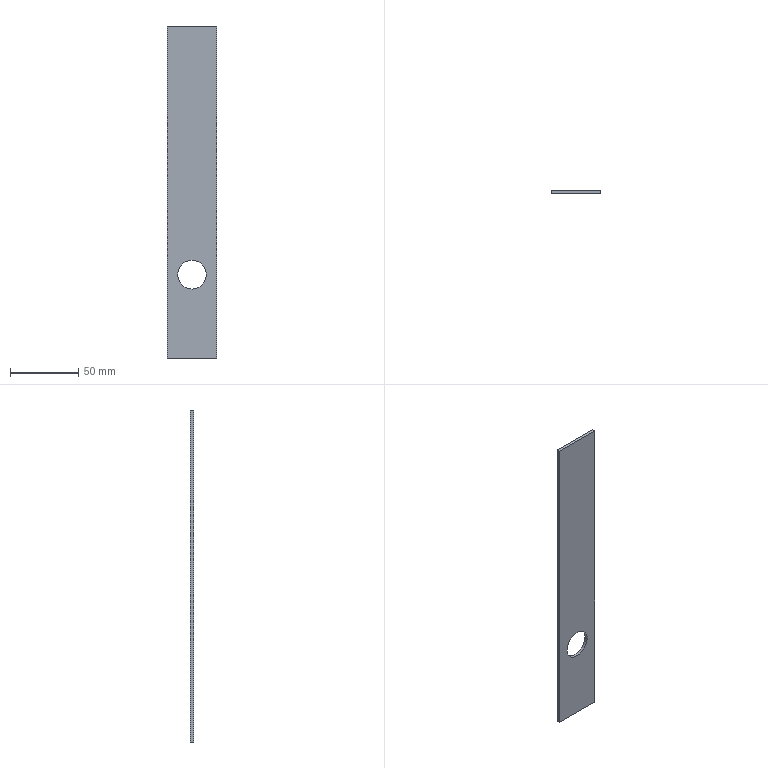Part | SolidWorks | features FlatPattern 1, SMBaseFlange 1, SheetMetal 1 | 1 solid | 8 faces | box 36.4 x 2.3 x 243 mm | volume 19547 mm3 | plane 6 | cylinder 2 | commonest cylinder face diameters 21 x2
STEP:
#1=CARTESIAN_POINT('',(0.,2.3,-71.));
#2=VERTEX_POINT('',#1);
#3=CARTESIAN_POINT('',(0.,2.3,-50.));
#4=VERTEX_POINT('',#3);
#5=CARTESIAN_POINT('',(0.,2.3,-60.5));
#6=DIRECTION('',(0.,1.,0.));
#7=DIRECTION('',(0.,0.,1.));
#8=AXIS2_PLACEMENT_3D('',#5,#6,#7);
#9=CIRCLE('',#8,10.5);
#10=EDGE_CURVE('',#2,#4,#9,.T.);
#11=ORIENTED_EDGE('',*,*,#10,.T.);
#12=CARTESIAN_POINT('',(0.,0.,-50.));
#13=VERTEX_POINT('',#12);
#14=CARTESIAN_POINT('',(0.,2.3,-50.));
#15=DIRECTION('',(0.,-1.,0.));
#16=VECTOR('',#15,1000.);
#17=LINE('',#14,#16);
#18=EDGE_CURVE('',#4,#13,#17,.T.);
#19=ORIENTED_EDGE('',*,*,#18,.T.);
#20=CARTESIAN_POINT('',(0.,0.,-71.));
#21=VERTEX_POINT('',#20);
#22=CARTESIAN_POINT('',(0.,0.,-60.5));
#23=DIRECTION('',(0.,1.,0.));
#24=DIRECTION('',(0.,0.,1.));
#25=AXIS2_PLACEMENT_3D('',#22,#23,#24);
#26=CIRCLE('',#25,10.5);
#27=EDGE_CURVE('',#21,#13,#26,.T.);
#28=ORIENTED_EDGE('',*,*,#27,.F.);
#29=CARTESIAN_POINT('',(0.,2.3,-71.));
#30=DIRECTION('',(0.,-1.,0.));
#31=VECTOR('',#30,1000.);
#32=LINE('',#29,#31);
#33=EDGE_CURVE('',#2,#21,#32,.T.);
#34=ORIENTED_EDGE('',*,*,#33,.F.);
#35=EDGE_LOOP('',(#11,#19,#28,#34));
#36=FACE_OUTER_BOUND('',#35,.T.);
#37=CARTESIAN_POINT('',(0.,2.3,-60.5));
#38=DIRECTION('',(0.,-1.,0.));
#39=DIRECTION('',(0.,0.,-1.));
#40=AXIS2_PLACEMENT_3D('',#37,#38,#39);
#41=CYLINDRICAL_SURFACE('',#40,10.5);
#42=ADVANCED_FACE('',(#36),#41,.F.);
#43=CARTESIAN_POINT('',(18.2,2.3,121.5));
#44=VERTEX_POINT('',#43);
#45=CARTESIAN_POINT('',(18.2,2.3,-121.5));
#46=VERTEX_POINT('',#45);
#47=CARTESIAN_POINT('',(18.2,2.3,-121.5));
#48=DIRECTION('',(0.,0.,-1.));
#49=VECTOR('',#48,1000.);
#50=LINE('',#47,#49);
#51=EDGE_CURVE('',#44,#46,#50,.T.);
#52=ORIENTED_EDGE('',*,*,#51,.T.);
#53=CARTESIAN_POINT('',(-18.2,2.3,-121.5));
#54=VERTEX_POINT('',#53);
#55=CARTESIAN_POINT('',(-18.2,2.3,-121.5));
#56=DIRECTION('',(-1.,0.,0.));
#57=VECTOR('',#56,1000.);
#58=LINE('',#55,#57);
#59=EDGE_CURVE('',#46,#54,#58,.T.);
#60=ORIENTED_EDGE('',*,*,#59,.T.);
#61=CARTESIAN_POINT('',(-18.2,2.3,121.5));
#62=VERTEX_POINT('',#61);
#63=CARTESIAN_POINT('',(-18.2,2.3,-121.5));
#64=DIRECTION('',(0.,0.,1.));
#65=VECTOR('',#64,1000.);
#66=LINE('',#63,#65);
#67=EDGE_CURVE('',#54,#62,#66,.T.);
#68=ORIENTED_EDGE('',*,*,#67,.T.);
#69=CARTESIAN_POINT('',(-18.2,2.3,121.5));
#70=DIRECTION('',(1.,0.,0.));
#71=VECTOR('',#70,1000.);
#72=LINE('',#69,#71);
#73=EDGE_CURVE('',#62,#44,#72,.T.);
#74=ORIENTED_EDGE('',*,*,#73,.T.);
#75=EDGE_LOOP('',(#52,#60,#68,#74));
#76=FACE_OUTER_BOUND('',#75,.T.);
#77=ORIENTED_EDGE('',*,*,#10,.F.);
#78=CARTESIAN_POINT('',(0.,2.3,-60.5));
#79=DIRECTION('',(0.,1.,0.));
#80=DIRECTION('',(0.,0.,1.));
#81=AXIS2_PLACEMENT_3D('',#78,#79,#80);
#82=CIRCLE('',#81,10.5);
#83=EDGE_CURVE('',#4,#2,#82,.T.);
#84=ORIENTED_EDGE('',*,*,#83,.F.);
#85=EDGE_LOOP('',(#77,#84));
#86=FACE_BOUND('',#85,.T.);
#87=CARTESIAN_POINT('',(0.,2.3,0.));
#88=DIRECTION('',(0.,1.,0.));
#89=DIRECTION('',(0.,0.,1.));
#90=AXIS2_PLACEMENT_3D('',#87,#88,#89);
#91=PLANE('',#90);
#92=ADVANCED_FACE('',(#76,#86),#91,.T.);
#93=CARTESIAN_POINT('',(18.2,0.,121.5));
#94=VERTEX_POINT('',#93);
#95=CARTESIAN_POINT('',(18.2,0.,-121.5));
#96=VERTEX_POINT('',#95);
#97=CARTESIAN_POINT('',(18.2,0.,-121.5));
#98=DIRECTION('',(0.,0.,-1.));
#99=VECTOR('',#98,1000.);
#100=LINE('',#97,#99);
#101=EDGE_CURVE('',#94,#96,#100,.T.);
#102=ORIENTED_EDGE('',*,*,#101,.F.);
#103=CARTESIAN_POINT('',(-18.2,0.,121.5));
#104=VERTEX_POINT('',#103);
#105=CARTESIAN_POINT('',(-18.2,0.,121.5));
#106=DIRECTION('',(1.,0.,0.));
#107=VECTOR('',#106,1000.);
#108=LINE('',#105,#107);
#109=EDGE_CURVE('',#104,#94,#108,.T.);
#110=ORIENTED_EDGE('',*,*,#109,.F.);
#111=CARTESIAN_POINT('',(-18.2,0.,-121.5));
#112=VERTEX_POINT('',#111);
#113=CARTESIAN_POINT('',(-18.2,0.,-121.5));
#114=DIRECTION('',(0.,0.,1.));
#115=VECTOR('',#114,1000.);
#116=LINE('',#113,#115);
#117=EDGE_CURVE('',#112,#104,#116,.T.);
#118=ORIENTED_EDGE('',*,*,#117,.F.);
#119=CARTESIAN_POINT('',(-18.2,0.,-121.5));
#120=DIRECTION('',(-1.,0.,0.));
#121=VECTOR('',#120,1000.);
#122=LINE('',#119,#121);
#123=EDGE_CURVE('',#96,#112,#122,.T.);
#124=ORIENTED_EDGE('',*,*,#123,.F.);
#125=EDGE_LOOP('',(#102,#110,#118,#124));
#126=FACE_OUTER_BOUND('',#125,.T.);
#127=ORIENTED_EDGE('',*,*,#27,.T.);
#128=CARTESIAN_POINT('',(0.,0.,-60.5));
#129=DIRECTION('',(0.,1.,0.));
#130=DIRECTION('',(0.,0.,1.));
#131=AXIS2_PLACEMENT_3D('',#128,#129,#130);
#132=CIRCLE('',#131,10.5);
#133=EDGE_CURVE('',#13,#21,#132,.T.);
#134=ORIENTED_EDGE('',*,*,#133,.T.);
#135=EDGE_LOOP('',(#127,#134));
#136=FACE_BOUND('',#135,.T.);
#137=CARTESIAN_POINT('',(0.,0.,0.));
#138=DIRECTION('',(0.,1.,0.));
#139=DIRECTION('',(0.,0.,1.));
#140=AXIS2_PLACEMENT_3D('',#137,#138,#139);
#141=PLANE('',#140);
#142=ADVANCED_FACE('',(#126,#136),#141,.F.);
#143=ORIENTED_EDGE('',*,*,#101,.T.);
#144=CARTESIAN_POINT('',(18.2,2.3,-121.5));
#145=DIRECTION('',(0.,-1.,0.));
#146=VECTOR('',#145,1000.);
#147=LINE('',#144,#146);
#148=EDGE_CURVE('',#46,#96,#147,.T.);
#149=ORIENTED_EDGE('',*,*,#148,.F.);
#150=ORIENTED_EDGE('',*,*,#51,.F.);
#151=CARTESIAN_POINT('',(18.2,2.3,121.5));
#152=DIRECTION('',(0.,-1.,0.));
#153=VECTOR('',#152,1000.);
#154=LINE('',#151,#153);
#155=EDGE_CURVE('',#44,#94,#154,.T.);
#156=ORIENTED_EDGE('',*,*,#155,.T.);
#157=EDGE_LOOP('',(#143,#149,#150,#156));
#158=FACE_OUTER_BOUND('',#157,.T.);
#159=CARTESIAN_POINT('',(18.2,2.3,-121.5));
#160=DIRECTION('',(-1.,0.,0.));
#161=DIRECTION('',(0.,0.,1.));
#162=AXIS2_PLACEMENT_3D('',#159,#160,#161);
#163=PLANE('',#162);
#164=ADVANCED_FACE('',(#158),#163,.F.);
#165=ORIENTED_EDGE('',*,*,#123,.T.);
#166=CARTESIAN_POINT('',(-18.2,2.3,-121.5));
#167=DIRECTION('',(0.,-1.,0.));
#168=VECTOR('',#167,1000.);
#169=LINE('',#166,#168);
#170=EDGE_CURVE('',#54,#112,#169,.T.);
#171=ORIENTED_EDGE('',*,*,#170,.F.);
#172=ORIENTED_EDGE('',*,*,#59,.F.);
#173=ORIENTED_EDGE('',*,*,#148,.T.);
#174=EDGE_LOOP('',(#165,#171,#172,#173));
#175=FACE_OUTER_BOUND('',#174,.T.);
#176=CARTESIAN_POINT('',(-18.2,2.3,-121.5));
#177=DIRECTION('',(0.,0.,1.));
#178=DIRECTION('',(1.,0.,0.));
#179=AXIS2_PLACEMENT_3D('',#176,#177,#178);
#180=PLANE('',#179);
#181=ADVANCED_FACE('',(#175),#180,.F.);
#182=ORIENTED_EDGE('',*,*,#117,.T.);
#183=CARTESIAN_POINT('',(-18.2,2.3,121.5));
#184=DIRECTION('',(0.,-1.,0.));
#185=VECTOR('',#184,1000.);
#186=LINE('',#183,#185);
#187=EDGE_CURVE('',#62,#104,#186,.T.);
#188=ORIENTED_EDGE('',*,*,#187,.F.);
#189=ORIENTED_EDGE('',*,*,#67,.F.);
#190=ORIENTED_EDGE('',*,*,#170,.T.);
#191=EDGE_LOOP('',(#182,#188,#189,#190));
#192=FACE_OUTER_BOUND('',#191,.T.);
#193=CARTESIAN_POINT('',(-18.2,2.3,-121.5));
#194=DIRECTION('',(1.,0.,0.));
#195=DIRECTION('',(0.,0.,-1.));
#196=AXIS2_PLACEMENT_3D('',#193,#194,#195);
#197=PLANE('',#196);
#198=ADVANCED_FACE('',(#192),#197,.F.);
#199=ORIENTED_EDGE('',*,*,#109,.T.);
#200=ORIENTED_EDGE('',*,*,#155,.F.);
#201=ORIENTED_EDGE('',*,*,#73,.F.);
#202=ORIENTED_EDGE('',*,*,#187,.T.);
#203=EDGE_LOOP('',(#199,#200,#201,#202));
#204=FACE_OUTER_BOUND('',#203,.T.);
#205=CARTESIAN_POINT('',(-18.2,2.3,121.5));
#206=DIRECTION('',(0.,0.,-1.));
#207=DIRECTION('',(-1.,0.,0.));
#208=AXIS2_PLACEMENT_3D('',#205,#206,#207);
#209=PLANE('',#208);
#210=ADVANCED_FACE('',(#204),#209,.F.);
#211=ORIENTED_EDGE('',*,*,#18,.F.);
#212=ORIENTED_EDGE('',*,*,#83,.T.);
#213=ORIENTED_EDGE('',*,*,#33,.T.);
#214=ORIENTED_EDGE('',*,*,#133,.F.);
#215=EDGE_LOOP('',(#211,#212,#213,#214));
#216=FACE_OUTER_BOUND('',#215,.T.);
#217=CARTESIAN_POINT('',(0.,2.3,-60.5));
#218=DIRECTION('',(0.,-1.,0.));
#219=DIRECTION('',(0.,0.,-1.));
#220=AXIS2_PLACEMENT_3D('',#217,#218,#219);
#221=CYLINDRICAL_SURFACE('',#220,10.5);
#222=ADVANCED_FACE('',(#216),#221,.F.);
#223=CLOSED_SHELL('',(#42,#92,#142,#164,#181,#198,#210,#222));
#224=MANIFOLD_SOLID_BREP('',#223);
#225=CARTESIAN_POINT('',(0.,0.,0.));
#226=DIRECTION('',(0.,0.,1.));
#227=DIRECTION('',(1.,0.,0.));
#228=AXIS2_PLACEMENT_3D('',#225,#226,#227);
#229=(LENGTH_UNIT()NAMED_UNIT(*)SI_UNIT(.MILLI.,.METRE.));
#230=UNCERTAINTY_MEASURE_WITH_UNIT(LENGTH_MEASURE(0.00001),#229,'','');
#231=(NAMED_UNIT(*)PLANE_ANGLE_UNIT()SI_UNIT($,.RADIAN.));
#232=(NAMED_UNIT(*)SI_UNIT($,.STERADIAN.)SOLID_ANGLE_UNIT());
#233=(GEOMETRIC_REPRESENTATION_CONTEXT(3)GLOBAL_UNCERTAINTY_ASSIGNED_CONTEXT((#230))GLOBAL_UNIT_ASSIGNED_CONTEXT((#229,#231,#232))REPRESENTATION_CONTEXT('',''));
#234=ADVANCED_BREP_SHAPE_REPRESENTATION('',(#224,#228),#233);